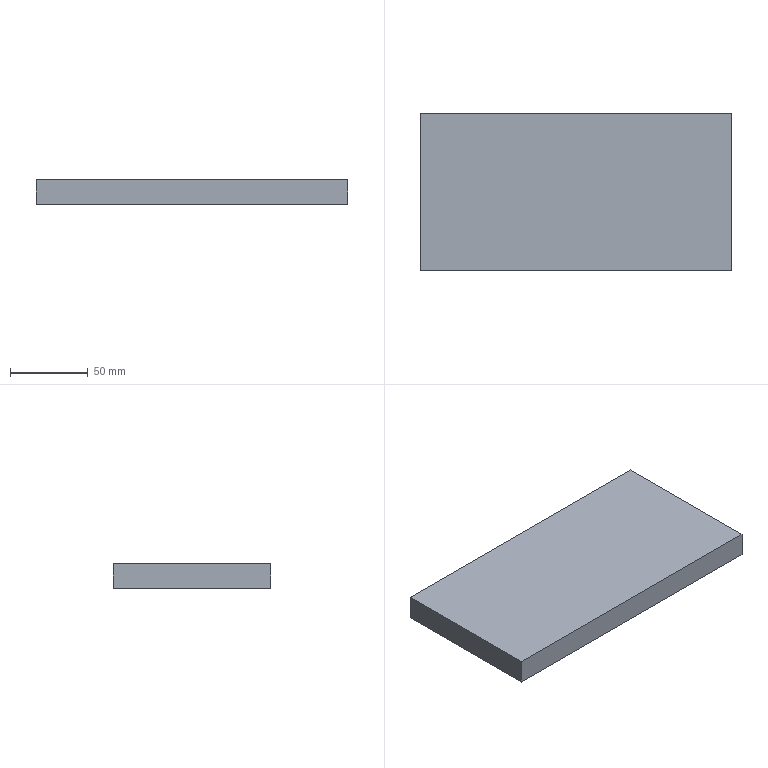Part | SolidWorks | features Extrusion 1 | 1 solid | 6 faces | box 200 x 101 x 16 mm | volume 323200 mm3 | plane 6
STEP:
#1=CARTESIAN_POINT('',(-100.,50.5,-8.));
#2=VERTEX_POINT('',#1);
#3=CARTESIAN_POINT('',(-100.,-50.5,-8.));
#4=VERTEX_POINT('',#3);
#5=CARTESIAN_POINT('',(-100.,-50.5,-8.));
#6=DIRECTION('',(0.,-1.,0.));
#7=VECTOR('',#6,1000.);
#8=LINE('',#5,#7);
#9=EDGE_CURVE('',#2,#4,#8,.T.);
#10=ORIENTED_EDGE('',*,*,#9,.T.);
#11=CARTESIAN_POINT('',(-100.,-50.5,8.));
#12=VERTEX_POINT('',#11);
#13=CARTESIAN_POINT('',(-100.,-50.5,8.));
#14=DIRECTION('',(0.,0.,-1.));
#15=VECTOR('',#14,1000.);
#16=LINE('',#13,#15);
#17=EDGE_CURVE('',#12,#4,#16,.T.);
#18=ORIENTED_EDGE('',*,*,#17,.F.);
#19=CARTESIAN_POINT('',(-100.,50.5,8.));
#20=VERTEX_POINT('',#19);
#21=CARTESIAN_POINT('',(-100.,-50.5,8.));
#22=DIRECTION('',(0.,-1.,0.));
#23=VECTOR('',#22,1000.);
#24=LINE('',#21,#23);
#25=EDGE_CURVE('',#20,#12,#24,.T.);
#26=ORIENTED_EDGE('',*,*,#25,.F.);
#27=CARTESIAN_POINT('',(-100.,50.5,8.));
#28=DIRECTION('',(0.,0.,-1.));
#29=VECTOR('',#28,1000.);
#30=LINE('',#27,#29);
#31=EDGE_CURVE('',#20,#2,#30,.T.);
#32=ORIENTED_EDGE('',*,*,#31,.T.);
#33=EDGE_LOOP('',(#10,#18,#26,#32));
#34=FACE_OUTER_BOUND('',#33,.T.);
#35=CARTESIAN_POINT('',(-100.,-50.5,8.));
#36=DIRECTION('',(1.,0.,0.));
#37=DIRECTION('',(0.,0.,-1.));
#38=AXIS2_PLACEMENT_3D('',#35,#36,#37);
#39=PLANE('',#38);
#40=ADVANCED_FACE('',(#34),#39,.F.);
#41=CARTESIAN_POINT('',(100.,-50.5,-8.));
#42=VERTEX_POINT('',#41);
#43=CARTESIAN_POINT('',(100.,-50.5,-8.));
#44=DIRECTION('',(1.,0.,0.));
#45=VECTOR('',#44,1000.);
#46=LINE('',#43,#45);
#47=EDGE_CURVE('',#4,#42,#46,.T.);
#48=ORIENTED_EDGE('',*,*,#47,.T.);
#49=CARTESIAN_POINT('',(100.,-50.5,8.));
#50=VERTEX_POINT('',#49);
#51=CARTESIAN_POINT('',(100.,-50.5,8.));
#52=DIRECTION('',(0.,0.,-1.));
#53=VECTOR('',#52,1000.);
#54=LINE('',#51,#53);
#55=EDGE_CURVE('',#50,#42,#54,.T.);
#56=ORIENTED_EDGE('',*,*,#55,.F.);
#57=CARTESIAN_POINT('',(100.,-50.5,8.));
#58=DIRECTION('',(1.,0.,0.));
#59=VECTOR('',#58,1000.);
#60=LINE('',#57,#59);
#61=EDGE_CURVE('',#12,#50,#60,.T.);
#62=ORIENTED_EDGE('',*,*,#61,.F.);
#63=ORIENTED_EDGE('',*,*,#17,.T.);
#64=EDGE_LOOP('',(#48,#56,#62,#63));
#65=FACE_OUTER_BOUND('',#64,.T.);
#66=CARTESIAN_POINT('',(100.,-50.5,8.));
#67=DIRECTION('',(0.,1.,0.));
#68=DIRECTION('',(-1.,0.,0.));
#69=AXIS2_PLACEMENT_3D('',#66,#67,#68);
#70=PLANE('',#69);
#71=ADVANCED_FACE('',(#65),#70,.F.);
#72=CARTESIAN_POINT('',(100.,50.5,-8.));
#73=VERTEX_POINT('',#72);
#74=CARTESIAN_POINT('',(100.,-50.5,-8.));
#75=DIRECTION('',(0.,1.,0.));
#76=VECTOR('',#75,1000.);
#77=LINE('',#74,#76);
#78=EDGE_CURVE('',#42,#73,#77,.T.);
#79=ORIENTED_EDGE('',*,*,#78,.T.);
#80=CARTESIAN_POINT('',(100.,50.5,8.));
#81=VERTEX_POINT('',#80);
#82=CARTESIAN_POINT('',(100.,50.5,8.));
#83=DIRECTION('',(0.,0.,-1.));
#84=VECTOR('',#83,1000.);
#85=LINE('',#82,#84);
#86=EDGE_CURVE('',#81,#73,#85,.T.);
#87=ORIENTED_EDGE('',*,*,#86,.F.);
#88=CARTESIAN_POINT('',(100.,-50.5,8.));
#89=DIRECTION('',(0.,1.,0.));
#90=VECTOR('',#89,1000.);
#91=LINE('',#88,#90);
#92=EDGE_CURVE('',#50,#81,#91,.T.);
#93=ORIENTED_EDGE('',*,*,#92,.F.);
#94=ORIENTED_EDGE('',*,*,#55,.T.);
#95=EDGE_LOOP('',(#79,#87,#93,#94));
#96=FACE_OUTER_BOUND('',#95,.T.);
#97=CARTESIAN_POINT('',(100.,-50.5,8.));
#98=DIRECTION('',(-1.,0.,0.));
#99=DIRECTION('',(0.,0.,1.));
#100=AXIS2_PLACEMENT_3D('',#97,#98,#99);
#101=PLANE('',#100);
#102=ADVANCED_FACE('',(#96),#101,.F.);
#103=CARTESIAN_POINT('',(100.,50.5,-8.));
#104=DIRECTION('',(-1.,0.,0.));
#105=VECTOR('',#104,1000.);
#106=LINE('',#103,#105);
#107=EDGE_CURVE('',#73,#2,#106,.T.);
#108=ORIENTED_EDGE('',*,*,#107,.T.);
#109=ORIENTED_EDGE('',*,*,#31,.F.);
#110=CARTESIAN_POINT('',(100.,50.5,8.));
#111=DIRECTION('',(-1.,0.,0.));
#112=VECTOR('',#111,1000.);
#113=LINE('',#110,#112);
#114=EDGE_CURVE('',#81,#20,#113,.T.);
#115=ORIENTED_EDGE('',*,*,#114,.F.);
#116=ORIENTED_EDGE('',*,*,#86,.T.);
#117=EDGE_LOOP('',(#108,#109,#115,#116));
#118=FACE_OUTER_BOUND('',#117,.T.);
#119=CARTESIAN_POINT('',(100.,50.5,8.));
#120=DIRECTION('',(0.,-1.,0.));
#121=DIRECTION('',(1.,0.,0.));
#122=AXIS2_PLACEMENT_3D('',#119,#120,#121);
#123=PLANE('',#122);
#124=ADVANCED_FACE('',(#118),#123,.F.);
#125=ORIENTED_EDGE('',*,*,#25,.T.);
#126=ORIENTED_EDGE('',*,*,#61,.T.);
#127=ORIENTED_EDGE('',*,*,#92,.T.);
#128=ORIENTED_EDGE('',*,*,#114,.T.);
#129=EDGE_LOOP('',(#125,#126,#127,#128));
#130=FACE_OUTER_BOUND('',#129,.T.);
#131=CARTESIAN_POINT('',(0.,0.,8.));
#132=DIRECTION('',(0.,0.,1.));
#133=DIRECTION('',(1.,0.,0.));
#134=AXIS2_PLACEMENT_3D('',#131,#132,#133);
#135=PLANE('',#134);
#136=ADVANCED_FACE('',(#130),#135,.T.);
#137=ORIENTED_EDGE('',*,*,#9,.F.);
#138=ORIENTED_EDGE('',*,*,#107,.F.);
#139=ORIENTED_EDGE('',*,*,#78,.F.);
#140=ORIENTED_EDGE('',*,*,#47,.F.);
#141=EDGE_LOOP('',(#137,#138,#139,#140));
#142=FACE_OUTER_BOUND('',#141,.T.);
#143=CARTESIAN_POINT('',(0.,0.,-8.));
#144=DIRECTION('',(0.,0.,1.));
#145=DIRECTION('',(1.,0.,0.));
#146=AXIS2_PLACEMENT_3D('',#143,#144,#145);
#147=PLANE('',#146);
#148=ADVANCED_FACE('',(#142),#147,.F.);
#149=CLOSED_SHELL('',(#40,#71,#102,#124,#136,#148));
#150=MANIFOLD_SOLID_BREP('',#149);
#151=CARTESIAN_POINT('',(0.,0.,0.));
#152=DIRECTION('',(0.,0.,1.));
#153=DIRECTION('',(1.,0.,0.));
#154=AXIS2_PLACEMENT_3D('',#151,#152,#153);
#155=(LENGTH_UNIT()NAMED_UNIT(*)SI_UNIT(.MILLI.,.METRE.));
#156=UNCERTAINTY_MEASURE_WITH_UNIT(LENGTH_MEASURE(0.00001),#155,'','');
#157=(NAMED_UNIT(*)PLANE_ANGLE_UNIT()SI_UNIT($,.RADIAN.));
#158=(NAMED_UNIT(*)SI_UNIT($,.STERADIAN.)SOLID_ANGLE_UNIT());
#159=(GEOMETRIC_REPRESENTATION_CONTEXT(3)GLOBAL_UNCERTAINTY_ASSIGNED_CONTEXT((#156))GLOBAL_UNIT_ASSIGNED_CONTEXT((#155,#157,#158))REPRESENTATION_CONTEXT('',''));
#160=ADVANCED_BREP_SHAPE_REPRESENTATION('',(#150,#154),#159);